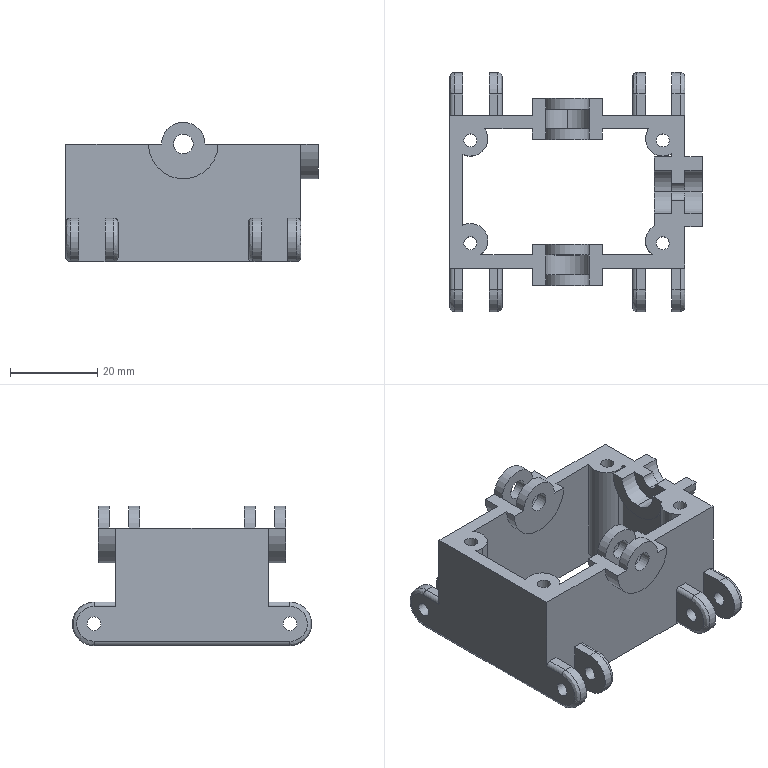Part | STEP file | 1 solid | 122 faces | box 58 x 55 x 32 mm | volume 19800 mm3 | cylinder 66 | plane 48 | spline 8 | commonest cylinder face diameters 10 x19 2 x14 16 x9 3.15 x8 8 x6 3 x4